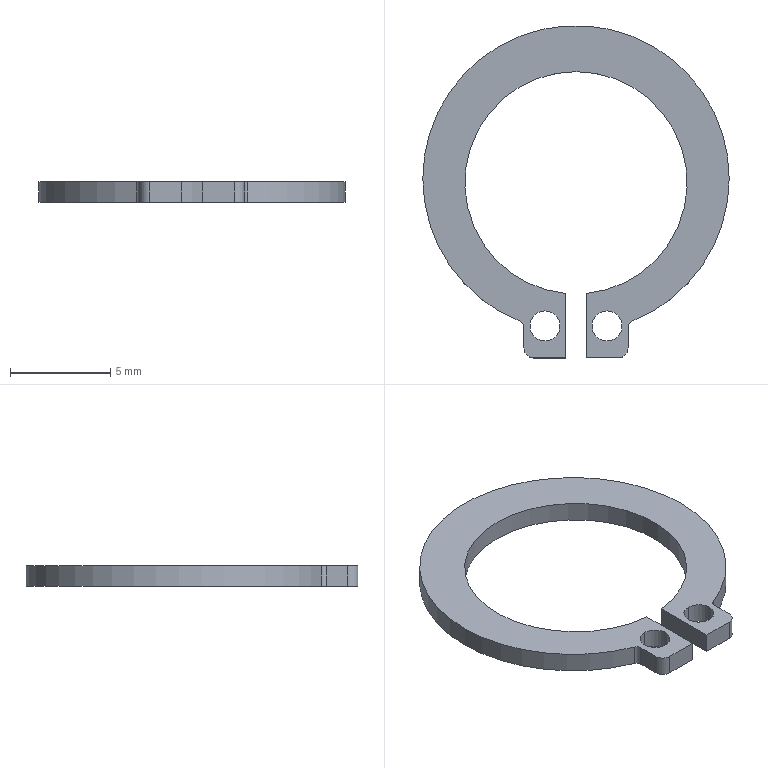Part | SolidWorks | features BaseBody 1 | 1 solid | 18 faces | box 15.3 x 16.6 x 1 mm | volume 87.791 mm3 | cylinder 10 | plane 8 | commonest cylinder face diameters 1.5 x4 0.6 x2 1 x2 11.1 x1 15.3 x1
STEP:
#1=CARTESIAN_POINT('',(-1.55,-6.4,0.));
#2=VERTEX_POINT('',#1);
#3=CARTESIAN_POINT('',(-1.55,-7.9,0.));
#4=VERTEX_POINT('',#3);
#5=CARTESIAN_POINT('',(-1.55,-7.15,0.));
#6=DIRECTION('',(0.,0.,1.));
#7=DIRECTION('',(0.,-1.,0.));
#8=AXIS2_PLACEMENT_3D('',#5,#6,#7);
#9=CIRCLE('',#8,0.75);
#10=EDGE_CURVE('',#2,#4,#9,.T.);
#11=ORIENTED_EDGE('',*,*,#10,.F.);
#12=CARTESIAN_POINT('',(-1.55,-6.4,1.));
#13=VERTEX_POINT('',#12);
#14=CARTESIAN_POINT('',(-1.55,-6.4,1.));
#15=DIRECTION('',(0.,0.,1.));
#16=VECTOR('',#15,1000.);
#17=LINE('',#14,#16);
#18=EDGE_CURVE('',#2,#13,#17,.T.);
#19=ORIENTED_EDGE('',*,*,#18,.T.);
#20=CARTESIAN_POINT('',(-1.55,-7.9,1.));
#21=VERTEX_POINT('',#20);
#22=CARTESIAN_POINT('',(-1.55,-7.15,1.));
#23=DIRECTION('',(0.,0.,-1.));
#24=DIRECTION('',(0.,-1.,0.));
#25=AXIS2_PLACEMENT_3D('',#22,#23,#24);
#26=CIRCLE('',#25,0.75);
#27=EDGE_CURVE('',#21,#13,#26,.T.);
#28=ORIENTED_EDGE('',*,*,#27,.F.);
#29=CARTESIAN_POINT('',(-1.55,-7.9,1.));
#30=DIRECTION('',(0.,0.,1.));
#31=VECTOR('',#30,1000.);
#32=LINE('',#29,#31);
#33=EDGE_CURVE('',#4,#21,#32,.T.);
#34=ORIENTED_EDGE('',*,*,#33,.F.);
#35=EDGE_LOOP('',(#11,#19,#28,#34));
#36=FACE_OUTER_BOUND('',#35,.T.);
#37=CARTESIAN_POINT('',(-1.55,-7.15,1.));
#38=DIRECTION('',(0.,0.,1.));
#39=DIRECTION('',(0.,-1.,0.));
#40=AXIS2_PLACEMENT_3D('',#37,#38,#39);
#41=CYLINDRICAL_SURFACE('',#40,0.75);
#42=ADVANCED_FACE('',(#36),#41,.F.);
#43=CARTESIAN_POINT('',(1.55,-6.4,0.));
#44=VERTEX_POINT('',#43);
#45=CARTESIAN_POINT('',(1.55,-7.9,0.));
#46=VERTEX_POINT('',#45);
#47=CARTESIAN_POINT('',(1.55,-7.15,0.));
#48=DIRECTION('',(0.,0.,1.));
#49=DIRECTION('',(0.,-1.,0.));
#50=AXIS2_PLACEMENT_3D('',#47,#48,#49);
#51=CIRCLE('',#50,0.75);
#52=EDGE_CURVE('',#44,#46,#51,.T.);
#53=ORIENTED_EDGE('',*,*,#52,.F.);
#54=CARTESIAN_POINT('',(1.55,-6.4,1.));
#55=VERTEX_POINT('',#54);
#56=CARTESIAN_POINT('',(1.55,-6.4,1.));
#57=DIRECTION('',(0.,0.,1.));
#58=VECTOR('',#57,1000.);
#59=LINE('',#56,#58);
#60=EDGE_CURVE('',#44,#55,#59,.T.);
#61=ORIENTED_EDGE('',*,*,#60,.T.);
#62=CARTESIAN_POINT('',(1.55,-7.9,1.));
#63=VERTEX_POINT('',#62);
#64=CARTESIAN_POINT('',(1.55,-7.15,1.));
#65=DIRECTION('',(0.,0.,-1.));
#66=DIRECTION('',(0.,-1.,0.));
#67=AXIS2_PLACEMENT_3D('',#64,#65,#66);
#68=CIRCLE('',#67,0.75);
#69=EDGE_CURVE('',#63,#55,#68,.T.);
#70=ORIENTED_EDGE('',*,*,#69,.F.);
#71=CARTESIAN_POINT('',(1.55,-7.9,1.));
#72=DIRECTION('',(0.,0.,1.));
#73=VECTOR('',#72,1000.);
#74=LINE('',#71,#73);
#75=EDGE_CURVE('',#46,#63,#74,.T.);
#76=ORIENTED_EDGE('',*,*,#75,.F.);
#77=EDGE_LOOP('',(#53,#61,#70,#76));
#78=FACE_OUTER_BOUND('',#77,.T.);
#79=CARTESIAN_POINT('',(1.55,-7.15,1.));
#80=DIRECTION('',(0.,0.,1.));
#81=DIRECTION('',(0.,-1.,0.));
#82=AXIS2_PLACEMENT_3D('',#79,#80,#81);
#83=CYLINDRICAL_SURFACE('',#82,0.75);
#84=ADVANCED_FACE('',(#78),#83,.F.);
#85=ORIENTED_EDGE('',*,*,#27,.T.);
#86=CARTESIAN_POINT('',(-1.55,-7.15,1.));
#87=DIRECTION('',(0.,0.,-1.));
#88=DIRECTION('',(0.,-1.,0.));
#89=AXIS2_PLACEMENT_3D('',#86,#87,#88);
#90=CIRCLE('',#89,0.75);
#91=EDGE_CURVE('',#13,#21,#90,.T.);
#92=ORIENTED_EDGE('',*,*,#91,.T.);
#93=EDGE_LOOP('',(#85,#92));
#94=FACE_BOUND('',#93,.T.);
#95=CARTESIAN_POINT('',(0.5,-5.527,1.));
#96=VERTEX_POINT('',#95);
#97=CARTESIAN_POINT('',(0.5,-8.75,1.));
#98=VERTEX_POINT('',#97);
#99=CARTESIAN_POINT('',(0.5,-7.202,1.));
#100=DIRECTION('',(0.,-1.,0.));
#101=VECTOR('',#100,1000.);
#102=LINE('',#99,#101);
#103=EDGE_CURVE('',#96,#98,#102,.T.);
#104=ORIENTED_EDGE('',*,*,#103,.T.);
#105=CARTESIAN_POINT('',(2.1,-8.75,1.));
#106=VERTEX_POINT('',#105);
#107=CARTESIAN_POINT('',(2.9,-8.75,1.));
#108=DIRECTION('',(1.,0.,0.));
#109=VECTOR('',#108,1000.);
#110=LINE('',#107,#109);
#111=EDGE_CURVE('',#98,#106,#110,.T.);
#112=ORIENTED_EDGE('',*,*,#111,.T.);
#113=CARTESIAN_POINT('',(2.6,-8.25,1.));
#114=VERTEX_POINT('',#113);
#115=CARTESIAN_POINT('',(2.1,-8.25,1.));
#116=DIRECTION('',(0.,0.,1.));
#117=DIRECTION('',(0.,-1.,0.));
#118=AXIS2_PLACEMENT_3D('',#115,#116,#117);
#119=CIRCLE('',#118,0.5);
#120=EDGE_CURVE('',#106,#114,#119,.T.);
#121=ORIENTED_EDGE('',*,*,#120,.T.);
#122=CARTESIAN_POINT('',(2.6,-7.202,1.));
#123=VERTEX_POINT('',#122);
#124=CARTESIAN_POINT('',(2.6,-7.202,1.));
#125=DIRECTION('',(0.,1.,0.));
#126=VECTOR('',#125,1000.);
#127=LINE('',#124,#126);
#128=EDGE_CURVE('',#114,#123,#127,.T.);
#129=ORIENTED_EDGE('',*,*,#128,.T.);
#130=CARTESIAN_POINT('',(2.791,-6.923,1.));
#131=VERTEX_POINT('',#130);
#132=CARTESIAN_POINT('',(2.9,-7.202,1.));
#133=DIRECTION('',(0.,0.,-1.));
#134=DIRECTION('',(0.,-1.,0.));
#135=AXIS2_PLACEMENT_3D('',#132,#133,#134);
#136=CIRCLE('',#135,0.3);
#137=EDGE_CURVE('',#123,#131,#136,.T.);
#138=ORIENTED_EDGE('',*,*,#137,.T.);
#139=CARTESIAN_POINT('',(-2.791,-6.923,1.));
#140=VERTEX_POINT('',#139);
#141=CARTESIAN_POINT('',(0.,0.2,1.));
#142=DIRECTION('',(0.,0.,1.));
#143=DIRECTION('',(0.,-1.,0.));
#144=AXIS2_PLACEMENT_3D('',#141,#142,#143);
#145=CIRCLE('',#144,7.65);
#146=EDGE_CURVE('',#131,#140,#145,.T.);
#147=ORIENTED_EDGE('',*,*,#146,.T.);
#148=CARTESIAN_POINT('',(-2.6,-7.202,1.));
#149=VERTEX_POINT('',#148);
#150=CARTESIAN_POINT('',(-2.9,-7.202,1.));
#151=DIRECTION('',(0.,0.,-1.));
#152=DIRECTION('',(0.,-1.,0.));
#153=AXIS2_PLACEMENT_3D('',#150,#151,#152);
#154=CIRCLE('',#153,0.3);
#155=EDGE_CURVE('',#140,#149,#154,.T.);
#156=ORIENTED_EDGE('',*,*,#155,.T.);
#157=CARTESIAN_POINT('',(-2.6,-8.25,1.));
#158=VERTEX_POINT('',#157);
#159=CARTESIAN_POINT('',(-2.6,-7.202,1.));
#160=DIRECTION('',(0.,-1.,0.));
#161=VECTOR('',#160,1000.);
#162=LINE('',#159,#161);
#163=EDGE_CURVE('',#149,#158,#162,.T.);
#164=ORIENTED_EDGE('',*,*,#163,.T.);
#165=CARTESIAN_POINT('',(-2.1,-8.75,1.));
#166=VERTEX_POINT('',#165);
#167=CARTESIAN_POINT('',(-2.1,-8.25,1.));
#168=DIRECTION('',(0.,0.,1.));
#169=DIRECTION('',(0.,-1.,0.));
#170=AXIS2_PLACEMENT_3D('',#167,#168,#169);
#171=CIRCLE('',#170,0.5);
#172=EDGE_CURVE('',#158,#166,#171,.T.);
#173=ORIENTED_EDGE('',*,*,#172,.T.);
#174=CARTESIAN_POINT('',(-0.5,-8.75,1.));
#175=VERTEX_POINT('',#174);
#176=CARTESIAN_POINT('',(2.9,-8.75,1.));
#177=DIRECTION('',(1.,0.,0.));
#178=VECTOR('',#177,1000.);
#179=LINE('',#176,#178);
#180=EDGE_CURVE('',#166,#175,#179,.T.);
#181=ORIENTED_EDGE('',*,*,#180,.T.);
#182=CARTESIAN_POINT('',(-0.5,-5.527,1.));
#183=VERTEX_POINT('',#182);
#184=CARTESIAN_POINT('',(-0.5,-7.202,1.));
#185=DIRECTION('',(0.,1.,0.));
#186=VECTOR('',#185,1000.);
#187=LINE('',#184,#186);
#188=EDGE_CURVE('',#175,#183,#187,.T.);
#189=ORIENTED_EDGE('',*,*,#188,.T.);
#190=CARTESIAN_POINT('',(0.,0.,1.));
#191=DIRECTION('',(0.,0.,-1.));
#192=DIRECTION('',(0.,-1.,0.));
#193=AXIS2_PLACEMENT_3D('',#190,#191,#192);
#194=CIRCLE('',#193,5.55);
#195=EDGE_CURVE('',#183,#96,#194,.T.);
#196=ORIENTED_EDGE('',*,*,#195,.T.);
#197=EDGE_LOOP('',(#104,#112,#121,#129,#138,#147,#156,#164,#173,#181,#189,#196));
#198=FACE_OUTER_BOUND('',#197,.T.);
#199=ORIENTED_EDGE('',*,*,#69,.T.);
#200=CARTESIAN_POINT('',(1.55,-7.15,1.));
#201=DIRECTION('',(0.,0.,-1.));
#202=DIRECTION('',(0.,-1.,0.));
#203=AXIS2_PLACEMENT_3D('',#200,#201,#202);
#204=CIRCLE('',#203,0.75);
#205=EDGE_CURVE('',#55,#63,#204,.T.);
#206=ORIENTED_EDGE('',*,*,#205,.T.);
#207=EDGE_LOOP('',(#199,#206));
#208=FACE_BOUND('',#207,.T.);
#209=CARTESIAN_POINT('',(2.9,-7.202,1.));
#210=DIRECTION('',(0.,0.,1.));
#211=DIRECTION('',(0.,-1.,0.));
#212=AXIS2_PLACEMENT_3D('',#209,#210,#211);
#213=PLANE('',#212);
#214=ADVANCED_FACE('',(#94,#198,#208),#213,.T.);
#215=ORIENTED_EDGE('',*,*,#18,.F.);
#216=CARTESIAN_POINT('',(-1.55,-7.15,0.));
#217=DIRECTION('',(0.,0.,1.));
#218=DIRECTION('',(0.,-1.,0.));
#219=AXIS2_PLACEMENT_3D('',#216,#217,#218);
#220=CIRCLE('',#219,0.75);
#221=EDGE_CURVE('',#4,#2,#220,.T.);
#222=ORIENTED_EDGE('',*,*,#221,.F.);
#223=ORIENTED_EDGE('',*,*,#33,.T.);
#224=ORIENTED_EDGE('',*,*,#91,.F.);
#225=EDGE_LOOP('',(#215,#222,#223,#224));
#226=FACE_OUTER_BOUND('',#225,.T.);
#227=CARTESIAN_POINT('',(-1.55,-7.15,1.));
#228=DIRECTION('',(0.,0.,1.));
#229=DIRECTION('',(0.,-1.,0.));
#230=AXIS2_PLACEMENT_3D('',#227,#228,#229);
#231=CYLINDRICAL_SURFACE('',#230,0.75);
#232=ADVANCED_FACE('',(#226),#231,.F.);
#233=ORIENTED_EDGE('',*,*,#111,.F.);
#234=CARTESIAN_POINT('',(0.5,-8.75,0.));
#235=VERTEX_POINT('',#234);
#236=CARTESIAN_POINT('',(0.5,-8.75,1.));
#237=DIRECTION('',(0.,0.,1.));
#238=VECTOR('',#237,1000.);
#239=LINE('',#236,#238);
#240=EDGE_CURVE('',#235,#98,#239,.T.);
#241=ORIENTED_EDGE('',*,*,#240,.F.);
#242=CARTESIAN_POINT('',(2.1,-8.75,0.));
#243=VERTEX_POINT('',#242);
#244=CARTESIAN_POINT('',(0.5,-8.75,0.));
#245=DIRECTION('',(-1.,0.,0.));
#246=VECTOR('',#245,1000.);
#247=LINE('',#244,#246);
#248=EDGE_CURVE('',#243,#235,#247,.T.);
#249=ORIENTED_EDGE('',*,*,#248,.F.);
#250=CARTESIAN_POINT('',(2.1,-8.75,1.));
#251=DIRECTION('',(0.,0.,-1.));
#252=VECTOR('',#251,1000.);
#253=LINE('',#250,#252);
#254=EDGE_CURVE('',#106,#243,#253,.T.);
#255=ORIENTED_EDGE('',*,*,#254,.F.);
#256=EDGE_LOOP('',(#233,#241,#249,#255));
#257=FACE_OUTER_BOUND('',#256,.T.);
#258=CARTESIAN_POINT('',(0.5,-8.75,1.));
#259=DIRECTION('',(0.,1.,0.));
#260=DIRECTION('',(-1.,0.,0.));
#261=AXIS2_PLACEMENT_3D('',#258,#259,#260);
#262=PLANE('',#261);
#263=ADVANCED_FACE('',(#257),#262,.F.);
#264=ORIENTED_EDGE('',*,*,#103,.F.);
#265=CARTESIAN_POINT('',(0.5,-5.527,0.));
#266=VERTEX_POINT('',#265);
#267=CARTESIAN_POINT('',(0.5,-5.527,1.));
#268=DIRECTION('',(0.,0.,1.));
#269=VECTOR('',#268,1000.);
#270=LINE('',#267,#269);
#271=EDGE_CURVE('',#266,#96,#270,.T.);
#272=ORIENTED_EDGE('',*,*,#271,.F.);
#273=CARTESIAN_POINT('',(0.5,-5.527,0.));
#274=DIRECTION('',(0.,1.,0.));
#275=VECTOR('',#274,1000.);
#276=LINE('',#273,#275);
#277=EDGE_CURVE('',#235,#266,#276,.T.);
#278=ORIENTED_EDGE('',*,*,#277,.F.);
#279=ORIENTED_EDGE('',*,*,#240,.T.);
#280=EDGE_LOOP('',(#264,#272,#278,#279));
#281=FACE_OUTER_BOUND('',#280,.T.);
#282=CARTESIAN_POINT('',(0.5,-5.527,1.));
#283=DIRECTION('',(1.,0.,0.));
#284=DIRECTION('',(0.,1.,0.));
#285=AXIS2_PLACEMENT_3D('',#282,#283,#284);
#286=PLANE('',#285);
#287=ADVANCED_FACE('',(#281),#286,.F.);
#288=CARTESIAN_POINT('',(-0.5,-5.527,0.));
#289=VERTEX_POINT('',#288);
#290=CARTESIAN_POINT('',(0.,0.,0.));
#291=DIRECTION('',(0.,0.,1.));
#292=DIRECTION('',(0.,-1.,0.));
#293=AXIS2_PLACEMENT_3D('',#290,#291,#292);
#294=CIRCLE('',#293,5.55);
#295=EDGE_CURVE('',#266,#289,#294,.T.);
#296=ORIENTED_EDGE('',*,*,#295,.F.);
#297=ORIENTED_EDGE('',*,*,#271,.T.);
#298=ORIENTED_EDGE('',*,*,#195,.F.);
#299=CARTESIAN_POINT('',(-0.5,-5.527,1.));
#300=DIRECTION('',(0.,0.,1.));
#301=VECTOR('',#300,1000.);
#302=LINE('',#299,#301);
#303=EDGE_CURVE('',#289,#183,#302,.T.);
#304=ORIENTED_EDGE('',*,*,#303,.F.);
#305=EDGE_LOOP('',(#296,#297,#298,#304));
#306=FACE_OUTER_BOUND('',#305,.T.);
#307=CARTESIAN_POINT('',(0.,0.,1.));
#308=DIRECTION('',(0.,0.,1.));
#309=DIRECTION('',(0.,-1.,0.));
#310=AXIS2_PLACEMENT_3D('',#307,#308,#309);
#311=CYLINDRICAL_SURFACE('',#310,5.55);
#312=ADVANCED_FACE('',(#306),#311,.F.);
#313=ORIENTED_EDGE('',*,*,#188,.F.);
#314=CARTESIAN_POINT('',(-0.5,-8.75,0.));
#315=VERTEX_POINT('',#314);
#316=CARTESIAN_POINT('',(-0.5,-8.75,1.));
#317=DIRECTION('',(0.,0.,1.));
#318=VECTOR('',#317,1000.);
#319=LINE('',#316,#318);
#320=EDGE_CURVE('',#315,#175,#319,.T.);
#321=ORIENTED_EDGE('',*,*,#320,.F.);
#322=CARTESIAN_POINT('',(-0.5,-8.75,0.));
#323=DIRECTION('',(0.,-1.,0.));
#324=VECTOR('',#323,1000.);
#325=LINE('',#322,#324);
#326=EDGE_CURVE('',#289,#315,#325,.T.);
#327=ORIENTED_EDGE('',*,*,#326,.F.);
#328=ORIENTED_EDGE('',*,*,#303,.T.);
#329=EDGE_LOOP('',(#313,#321,#327,#328));
#330=FACE_OUTER_BOUND('',#329,.T.);
#331=CARTESIAN_POINT('',(-0.5,-8.75,1.));
#332=DIRECTION('',(-1.,0.,0.));
#333=DIRECTION('',(0.,-1.,0.));
#334=AXIS2_PLACEMENT_3D('',#331,#332,#333);
#335=PLANE('',#334);
#336=ADVANCED_FACE('',(#330),#335,.F.);
#337=ORIENTED_EDGE('',*,*,#180,.F.);
#338=CARTESIAN_POINT('',(-2.1,-8.75,0.));
#339=VERTEX_POINT('',#338);
#340=CARTESIAN_POINT('',(-2.1,-8.75,1.));
#341=DIRECTION('',(0.,0.,1.));
#342=VECTOR('',#341,1000.);
#343=LINE('',#340,#342);
#344=EDGE_CURVE('',#339,#166,#343,.T.);
#345=ORIENTED_EDGE('',*,*,#344,.F.);
#346=CARTESIAN_POINT('',(-2.1,-8.75,0.));
#347=DIRECTION('',(-1.,0.,0.));
#348=VECTOR('',#347,1000.);
#349=LINE('',#346,#348);
#350=EDGE_CURVE('',#315,#339,#349,.T.);
#351=ORIENTED_EDGE('',*,*,#350,.F.);
#352=ORIENTED_EDGE('',*,*,#320,.T.);
#353=EDGE_LOOP('',(#337,#345,#351,#352));
#354=FACE_OUTER_BOUND('',#353,.T.);
#355=CARTESIAN_POINT('',(-2.1,-8.75,1.));
#356=DIRECTION('',(0.,1.,0.));
#357=DIRECTION('',(-1.,0.,0.));
#358=AXIS2_PLACEMENT_3D('',#355,#356,#357);
#359=PLANE('',#358);
#360=ADVANCED_FACE('',(#354),#359,.F.);
#361=CARTESIAN_POINT('',(-2.6,-8.25,0.));
#362=VERTEX_POINT('',#361);
#363=CARTESIAN_POINT('',(-2.1,-8.25,0.));
#364=DIRECTION('',(0.,0.,1.));
#365=DIRECTION('',(0.,-1.,0.));
#366=AXIS2_PLACEMENT_3D('',#363,#364,#365);
#367=CIRCLE('',#366,0.5);
#368=EDGE_CURVE('',#362,#339,#367,.T.);
#369=ORIENTED_EDGE('',*,*,#368,.T.);
#370=ORIENTED_EDGE('',*,*,#344,.T.);
#371=ORIENTED_EDGE('',*,*,#172,.F.);
#372=CARTESIAN_POINT('',(-2.6,-8.25,1.));
#373=DIRECTION('',(0.,0.,-1.));
#374=VECTOR('',#373,1000.);
#375=LINE('',#372,#374);
#376=EDGE_CURVE('',#158,#362,#375,.T.);
#377=ORIENTED_EDGE('',*,*,#376,.T.);
#378=EDGE_LOOP('',(#369,#370,#371,#377));
#379=FACE_OUTER_BOUND('',#378,.T.);
#380=CARTESIAN_POINT('',(-2.1,-8.25,1.));
#381=DIRECTION('',(0.,0.,1.));
#382=DIRECTION('',(0.,-1.,0.));
#383=AXIS2_PLACEMENT_3D('',#380,#381,#382);
#384=CYLINDRICAL_SURFACE('',#383,0.5);
#385=ADVANCED_FACE('',(#379),#384,.T.);
#386=ORIENTED_EDGE('',*,*,#163,.F.);
#387=CARTESIAN_POINT('',(-2.6,-7.202,0.));
#388=VERTEX_POINT('',#387);
#389=CARTESIAN_POINT('',(-2.6,-7.202,1.));
#390=DIRECTION('',(0.,0.,1.));
#391=VECTOR('',#390,1000.);
#392=LINE('',#389,#391);
#393=EDGE_CURVE('',#388,#149,#392,.T.);
#394=ORIENTED_EDGE('',*,*,#393,.F.);
#395=CARTESIAN_POINT('',(-2.6,-7.202,0.));
#396=DIRECTION('',(0.,1.,0.));
#397=VECTOR('',#396,1000.);
#398=LINE('',#395,#397);
#399=EDGE_CURVE('',#362,#388,#398,.T.);
#400=ORIENTED_EDGE('',*,*,#399,.F.);
#401=ORIENTED_EDGE('',*,*,#376,.F.);
#402=EDGE_LOOP('',(#386,#394,#400,#401));
#403=FACE_OUTER_BOUND('',#402,.T.);
#404=CARTESIAN_POINT('',(-2.6,-7.202,1.));
#405=DIRECTION('',(1.,0.,0.));
#406=DIRECTION('',(0.,1.,0.));
#407=AXIS2_PLACEMENT_3D('',#404,#405,#406);
#408=PLANE('',#407);
#409=ADVANCED_FACE('',(#403),#408,.F.);
#410=ORIENTED_EDGE('',*,*,#155,.F.);
#411=CARTESIAN_POINT('',(-2.791,-6.923,0.));
#412=VERTEX_POINT('',#411);
#413=CARTESIAN_POINT('',(-2.791,-6.923,1.));
#414=DIRECTION('',(0.,0.,1.));
#415=VECTOR('',#414,1000.);
#416=LINE('',#413,#415);
#417=EDGE_CURVE('',#412,#140,#416,.T.);
#418=ORIENTED_EDGE('',*,*,#417,.F.);
#419=CARTESIAN_POINT('',(-2.9,-7.202,0.));
#420=DIRECTION('',(0.,0.,1.));
#421=DIRECTION('',(0.,-1.,0.));
#422=AXIS2_PLACEMENT_3D('',#419,#420,#421);
#423=CIRCLE('',#422,0.3);
#424=EDGE_CURVE('',#388,#412,#423,.T.);
#425=ORIENTED_EDGE('',*,*,#424,.F.);
#426=ORIENTED_EDGE('',*,*,#393,.T.);
#427=EDGE_LOOP('',(#410,#418,#425,#426));
#428=FACE_OUTER_BOUND('',#427,.T.);
#429=CARTESIAN_POINT('',(-2.9,-7.202,1.));
#430=DIRECTION('',(0.,0.,1.));
#431=DIRECTION('',(0.,-1.,0.));
#432=AXIS2_PLACEMENT_3D('',#429,#430,#431);
#433=CYLINDRICAL_SURFACE('',#432,0.3);
#434=ADVANCED_FACE('',(#428),#433,.F.);
#435=ORIENTED_EDGE('',*,*,#417,.T.);
#436=ORIENTED_EDGE('',*,*,#146,.F.);
#437=CARTESIAN_POINT('',(2.791,-6.923,0.));
#438=VERTEX_POINT('',#437);
#439=CARTESIAN_POINT('',(2.791,-6.923,1.));
#440=DIRECTION('',(0.,0.,-1.));
#441=VECTOR('',#440,1000.);
#442=LINE('',#439,#441);
#443=EDGE_CURVE('',#131,#438,#442,.T.);
#444=ORIENTED_EDGE('',*,*,#443,.T.);
#445=CARTESIAN_POINT('',(0.,0.2,0.));
#446=DIRECTION('',(0.,0.,1.));
#447=DIRECTION('',(0.,-1.,0.));
#448=AXIS2_PLACEMENT_3D('',#445,#446,#447);
#449=CIRCLE('',#448,7.65);
#450=EDGE_CURVE('',#438,#412,#449,.T.);
#451=ORIENTED_EDGE('',*,*,#450,.T.);
#452=EDGE_LOOP('',(#435,#436,#444,#451));
#453=FACE_OUTER_BOUND('',#452,.T.);
#454=CARTESIAN_POINT('',(0.,0.2,1.));
#455=DIRECTION('',(0.,0.,1.));
#456=DIRECTION('',(0.,-1.,0.));
#457=AXIS2_PLACEMENT_3D('',#454,#455,#456);
#458=CYLINDRICAL_SURFACE('',#457,7.65);
#459=ADVANCED_FACE('',(#453),#458,.T.);
#460=ORIENTED_EDGE('',*,*,#137,.F.);
#461=CARTESIAN_POINT('',(2.6,-7.202,0.));
#462=VERTEX_POINT('',#461);
#463=CARTESIAN_POINT('',(2.6,-7.202,1.));
#464=DIRECTION('',(0.,0.,1.));
#465=VECTOR('',#464,1000.);
#466=LINE('',#463,#465);
#467=EDGE_CURVE('',#462,#123,#466,.T.);
#468=ORIENTED_EDGE('',*,*,#467,.F.);
#469=CARTESIAN_POINT('',(2.9,-7.202,0.));
#470=DIRECTION('',(0.,0.,1.));
#471=DIRECTION('',(0.,-1.,0.));
#472=AXIS2_PLACEMENT_3D('',#469,#470,#471);
#473=CIRCLE('',#472,0.3);
#474=EDGE_CURVE('',#438,#462,#473,.T.);
#475=ORIENTED_EDGE('',*,*,#474,.F.);
#476=ORIENTED_EDGE('',*,*,#443,.F.);
#477=EDGE_LOOP('',(#460,#468,#475,#476));
#478=FACE_OUTER_BOUND('',#477,.T.);
#479=CARTESIAN_POINT('',(2.9,-7.202,1.));
#480=DIRECTION('',(0.,0.,1.));
#481=DIRECTION('',(0.,-1.,0.));
#482=AXIS2_PLACEMENT_3D('',#479,#480,#481);
#483=CYLINDRICAL_SURFACE('',#482,0.3);
#484=ADVANCED_FACE('',(#478),#483,.F.);
#485=ORIENTED_EDGE('',*,*,#128,.F.);
#486=CARTESIAN_POINT('',(2.6,-8.25,0.));
#487=VERTEX_POINT('',#486);
#488=CARTESIAN_POINT('',(2.6,-8.25,1.));
#489=DIRECTION('',(0.,0.,1.));
#490=VECTOR('',#489,1000.);
#491=LINE('',#488,#490);
#492=EDGE_CURVE('',#487,#114,#491,.T.);
#493=ORIENTED_EDGE('',*,*,#492,.F.);
#494=CARTESIAN_POINT('',(2.6,-8.25,0.));
#495=DIRECTION('',(0.,-1.,0.));
#496=VECTOR('',#495,1000.);
#497=LINE('',#494,#496);
#498=EDGE_CURVE('',#462,#487,#497,.T.);
#499=ORIENTED_EDGE('',*,*,#498,.F.);
#500=ORIENTED_EDGE('',*,*,#467,.T.);
#501=EDGE_LOOP('',(#485,#493,#499,#500));
#502=FACE_OUTER_BOUND('',#501,.T.);
#503=CARTESIAN_POINT('',(2.6,-8.25,1.));
#504=DIRECTION('',(-1.,0.,0.));
#505=DIRECTION('',(0.,-1.,0.));
#506=AXIS2_PLACEMENT_3D('',#503,#504,#505);
#507=PLANE('',#506);
#508=ADVANCED_FACE('',(#502),#507,.F.);
#509=CARTESIAN_POINT('',(2.1,-8.25,0.));
#510=DIRECTION('',(0.,0.,1.));
#511=DIRECTION('',(0.,-1.,0.));
#512=AXIS2_PLACEMENT_3D('',#509,#510,#511);
#513=CIRCLE('',#512,0.5);
#514=EDGE_CURVE('',#243,#487,#513,.T.);
#515=ORIENTED_EDGE('',*,*,#514,.T.);
#516=ORIENTED_EDGE('',*,*,#492,.T.);
#517=ORIENTED_EDGE('',*,*,#120,.F.);
#518=ORIENTED_EDGE('',*,*,#254,.T.);
#519=EDGE_LOOP('',(#515,#516,#517,#518));
#520=FACE_OUTER_BOUND('',#519,.T.);
#521=CARTESIAN_POINT('',(2.1,-8.25,1.));
#522=DIRECTION('',(0.,0.,1.));
#523=DIRECTION('',(0.,-1.,0.));
#524=AXIS2_PLACEMENT_3D('',#521,#522,#523);
#525=CYLINDRICAL_SURFACE('',#524,0.5);
#526=ADVANCED_FACE('',(#520),#525,.T.);
#527=ORIENTED_EDGE('',*,*,#60,.F.);
#528=CARTESIAN_POINT('',(1.55,-7.15,0.));
#529=DIRECTION('',(0.,0.,1.));
#530=DIRECTION('',(0.,-1.,0.));
#531=AXIS2_PLACEMENT_3D('',#528,#529,#530);
#532=CIRCLE('',#531,0.75);
#533=EDGE_CURVE('',#46,#44,#532,.T.);
#534=ORIENTED_EDGE('',*,*,#533,.F.);
#535=ORIENTED_EDGE('',*,*,#75,.T.);
#536=ORIENTED_EDGE('',*,*,#205,.F.);
#537=EDGE_LOOP('',(#527,#534,#535,#536));
#538=FACE_OUTER_BOUND('',#537,.T.);
#539=CARTESIAN_POINT('',(1.55,-7.15,1.));
#540=DIRECTION('',(0.,0.,1.));
#541=DIRECTION('',(0.,-1.,0.));
#542=AXIS2_PLACEMENT_3D('',#539,#540,#541);
#543=CYLINDRICAL_SURFACE('',#542,0.75);
#544=ADVANCED_FACE('',(#538),#543,.F.);
#545=ORIENTED_EDGE('',*,*,#221,.T.);
#546=ORIENTED_EDGE('',*,*,#10,.T.);
#547=EDGE_LOOP('',(#545,#546));
#548=FACE_BOUND('',#547,.T.);
#549=ORIENTED_EDGE('',*,*,#514,.F.);
#550=ORIENTED_EDGE('',*,*,#248,.T.);
#551=ORIENTED_EDGE('',*,*,#277,.T.);
#552=ORIENTED_EDGE('',*,*,#295,.T.);
#553=ORIENTED_EDGE('',*,*,#326,.T.);
#554=ORIENTED_EDGE('',*,*,#350,.T.);
#555=ORIENTED_EDGE('',*,*,#368,.F.);
#556=ORIENTED_EDGE('',*,*,#399,.T.);
#557=ORIENTED_EDGE('',*,*,#424,.T.);
#558=ORIENTED_EDGE('',*,*,#450,.F.);
#559=ORIENTED_EDGE('',*,*,#474,.T.);
#560=ORIENTED_EDGE('',*,*,#498,.T.);
#561=EDGE_LOOP('',(#549,#550,#551,#552,#553,#554,#555,#556,#557,#558,#559,#560));
#562=FACE_OUTER_BOUND('',#561,.T.);
#563=ORIENTED_EDGE('',*,*,#533,.T.);
#564=ORIENTED_EDGE('',*,*,#52,.T.);
#565=EDGE_LOOP('',(#563,#564));
#566=FACE_BOUND('',#565,.T.);
#567=CARTESIAN_POINT('',(2.9,-7.202,0.));
#568=DIRECTION('',(0.,0.,1.));
#569=DIRECTION('',(0.,-1.,0.));
#570=AXIS2_PLACEMENT_3D('',#567,#568,#569);
#571=PLANE('',#570);
#572=ADVANCED_FACE('',(#548,#562,#566),#571,.F.);
#573=CLOSED_SHELL('',(#42,#84,#214,#232,#263,#287,#312,#336,#360,#385,#409,#434,#459,#484,#508,#526,#544,#572));
#574=MANIFOLD_SOLID_BREP('',#573);
#575=CARTESIAN_POINT('',(0.,0.,0.));
#576=DIRECTION('',(0.,0.,1.));
#577=DIRECTION('',(1.,0.,0.));
#578=AXIS2_PLACEMENT_3D('',#575,#576,#577);
#579=(LENGTH_UNIT()NAMED_UNIT(*)SI_UNIT(.MILLI.,.METRE.));
#580=UNCERTAINTY_MEASURE_WITH_UNIT(LENGTH_MEASURE(0.00001),#579,'','');
#581=(NAMED_UNIT(*)PLANE_ANGLE_UNIT()SI_UNIT($,.RADIAN.));
#582=(NAMED_UNIT(*)SI_UNIT($,.STERADIAN.)SOLID_ANGLE_UNIT());
#583=(GEOMETRIC_REPRESENTATION_CONTEXT(3)GLOBAL_UNCERTAINTY_ASSIGNED_CONTEXT((#580))GLOBAL_UNIT_ASSIGNED_CONTEXT((#579,#581,#582))REPRESENTATION_CONTEXT('',''));
#584=ADVANCED_BREP_SHAPE_REPRESENTATION('',(#574,#578),#583);